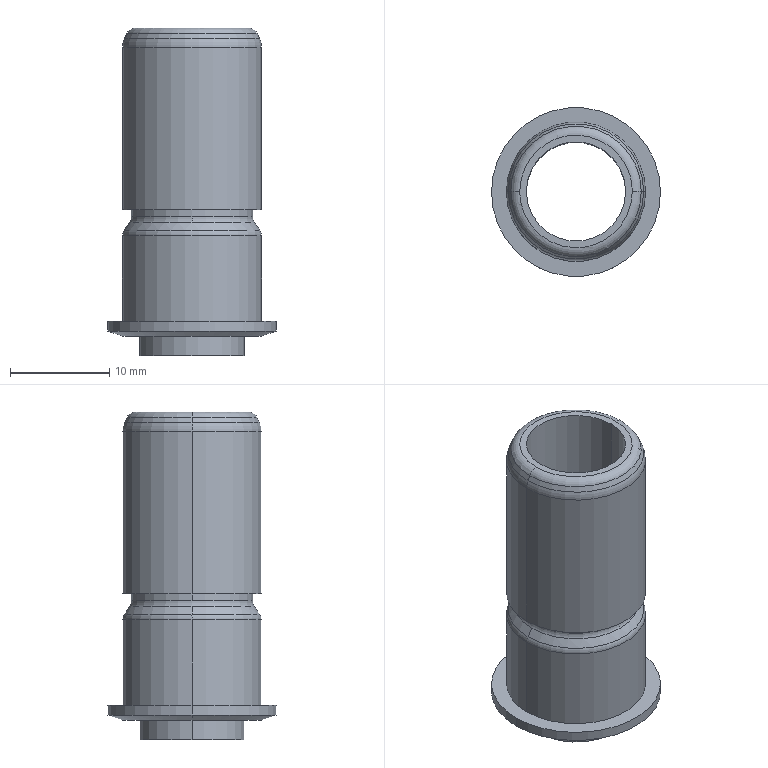Part | NX | features BREP 1 | 1 solid | 31 faces | box 17 x 17 x 33 mm | volume 2358 mm3 | cylinder 12 | torus 8 | cone 6 | plane 5 | commonest cylinder face diameters 14 x4 10 x2 10.5 x2 12.2 x2 17 x2
STEP:
#1=CARTESIAN_POINT('',(-514.52,233.142,1216.091));
#2=VERTEX_POINT('',#1);
#3=CARTESIAN_POINT('',(-524.52,233.142,1216.091));
#4=VERTEX_POINT('',#3);
#5=CARTESIAN_POINT('',(-519.52,233.142,1216.091));
#6=DIRECTION('',(0.,0.,-1.));
#7=DIRECTION('',(-1.,0.,0.));
#8=AXIS2_PLACEMENT_3D('',#5,#6,#7);
#9=CIRCLE('',#8,5.);
#10=EDGE_CURVE('',#2,#4,#9,.T.);
#11=ORIENTED_EDGE('',*,*,#10,.F.);
#12=CARTESIAN_POINT('',(-514.52,233.142,1183.091));
#13=VERTEX_POINT('',#12);
#14=CARTESIAN_POINT('',(-514.52,233.142,1216.091));
#15=DIRECTION('',(0.,0.,-1.));
#16=VECTOR('',#15,1000.);
#17=LINE('',#14,#16);
#18=EDGE_CURVE('',#13,#2,#17,.F.);
#19=ORIENTED_EDGE('',*,*,#18,.F.);
#20=CARTESIAN_POINT('',(-524.52,233.142,1183.091));
#21=VERTEX_POINT('',#20);
#22=CARTESIAN_POINT('',(-519.52,233.142,1183.091));
#23=DIRECTION('',(0.,0.,1.));
#24=DIRECTION('',(-1.,0.,0.));
#25=AXIS2_PLACEMENT_3D('',#22,#23,#24);
#26=CIRCLE('',#25,5.);
#27=EDGE_CURVE('',#21,#13,#26,.T.);
#28=ORIENTED_EDGE('',*,*,#27,.F.);
#29=CARTESIAN_POINT('',(-524.52,233.142,1216.091));
#30=DIRECTION('',(0.,0.,-1.));
#31=VECTOR('',#30,1000.);
#32=LINE('',#29,#31);
#33=EDGE_CURVE('',#21,#4,#32,.F.);
#34=ORIENTED_EDGE('',*,*,#33,.T.);
#35=EDGE_LOOP('',(#11,#19,#28,#34));
#36=FACE_BOUND('',#35,.T.);
#37=CARTESIAN_POINT('',(-519.52,233.142,1216.091));
#38=DIRECTION('',(0.,0.,-1.));
#39=DIRECTION('',(1.,0.,0.));
#40=AXIS2_PLACEMENT_3D('',#37,#38,#39);
#41=CYLINDRICAL_SURFACE('',#40,5.);
#42=ADVANCED_FACE('',(#36),#41,.F.);
#43=CARTESIAN_POINT('',(-512.95,233.142,1215.514));
#44=VERTEX_POINT('',#43);
#45=CARTESIAN_POINT('',(-526.089,233.142,1215.514));
#46=VERTEX_POINT('',#45);
#47=CARTESIAN_POINT('',(-519.52,233.142,1215.514));
#48=DIRECTION('',(0.,0.,1.));
#49=DIRECTION('',(0.01126,0.9999,0.));
#50=AXIS2_PLACEMENT_3D('',#47,#48,#49);
#51=CIRCLE('',#50,6.569);
#52=EDGE_CURVE('',#44,#46,#51,.T.);
#53=ORIENTED_EDGE('',*,*,#52,.T.);
#54=CARTESIAN_POINT('',(-525.182,233.142,1216.091));
#55=VERTEX_POINT('',#54);
#56=CARTESIAN_POINT('',(-525.182,233.142,1215.091));
#57=DIRECTION('',(0.,1.,0.));
#58=DIRECTION('',(0.,0.,1.));
#59=AXIS2_PLACEMENT_3D('',#56,#57,#58);
#60=CIRCLE('',#59,1.);
#61=EDGE_CURVE('',#46,#55,#60,.T.);
#62=ORIENTED_EDGE('',*,*,#61,.T.);
#63=CARTESIAN_POINT('',(-519.587,238.804,1216.091));
#64=VERTEX_POINT('',#63);
#65=CARTESIAN_POINT('',(-525.182,233.142,1216.091));
#66=CARTESIAN_POINT('',(-525.182,233.51,1216.091));
#67=CARTESIAN_POINT('',(-525.146,233.878,1216.091));
#68=CARTESIAN_POINT('',(-525.057,234.328,1216.091));
#69=CARTESIAN_POINT('',(-525.037,234.418,1216.091));
#70=CARTESIAN_POINT('',(-525.004,234.552,1216.091));
#71=CARTESIAN_POINT('',(-524.986,234.619,1216.091));
#72=CARTESIAN_POINT('',(-524.966,234.691,1216.091));
#73=CARTESIAN_POINT('',(-524.958,234.719,1216.091));
#74=CARTESIAN_POINT('',(-524.955,234.73,1216.091));
#75=CARTESIAN_POINT('',(-524.953,234.737,1216.091));
#76=CARTESIAN_POINT('',(-524.952,234.741,1216.091));
#77=CARTESIAN_POINT('',(-524.951,234.744,1216.091));
#78=CARTESIAN_POINT('',(-524.941,234.779,1216.091));
#79=CARTESIAN_POINT('',(-524.919,234.853,1216.091));
#80=CARTESIAN_POINT('',(-524.87,234.997,1216.091));
#81=CARTESIAN_POINT('',(-524.859,235.029,1216.091));
#82=CARTESIAN_POINT('',(-524.841,235.08,1216.091));
#83=CARTESIAN_POINT('',(-524.831,235.106,1216.091));
#84=CARTESIAN_POINT('',(-524.82,235.134,1216.091));
#85=CARTESIAN_POINT('',(-524.815,235.148,1216.091));
#86=CARTESIAN_POINT('',(-524.813,235.154,1216.091));
#87=CARTESIAN_POINT('',(-524.811,235.16,1216.091));
#88=CARTESIAN_POINT('',(-524.792,235.209,1216.091));
#89=CARTESIAN_POINT('',(-524.773,235.257,1216.091));
#90=CARTESIAN_POINT('',(-524.681,235.479,1216.091));
#91=CARTESIAN_POINT('',(-524.602,235.646,1216.091));
#92=CARTESIAN_POINT('',(-524.499,235.84,1216.091));
#93=CARTESIAN_POINT('',(-524.478,235.878,1216.091));
#94=CARTESIAN_POINT('',(-524.436,235.953,1216.091));
#95=CARTESIAN_POINT('',(-524.413,235.992,1216.091));
#96=CARTESIAN_POINT('',(-524.342,236.111,1216.091));
#97=CARTESIAN_POINT('',(-524.293,236.189,1216.091));
#98=CARTESIAN_POINT('',(-524.141,236.419,1216.091));
#99=CARTESIAN_POINT('',(-524.032,236.568,1216.091));
#100=CARTESIAN_POINT('',(-523.858,236.782,1216.091));
#101=CARTESIAN_POINT('',(-523.768,236.887,1216.091));
#102=CARTESIAN_POINT('',(-523.659,237.006,1216.091));
#103=CARTESIAN_POINT('',(-523.604,237.065,1216.091));
#104=CARTESIAN_POINT('',(-523.576,237.093,1216.091));
#105=CARTESIAN_POINT('',(-523.562,237.108,1216.091));
#106=CARTESIAN_POINT('',(-523.556,237.114,1216.091));
#107=CARTESIAN_POINT('',(-523.552,237.118,1216.091));
#108=CARTESIAN_POINT('',(-523.549,237.121,1216.091));
#109=CARTESIAN_POINT('',(-523.495,237.176,1216.091));
#110=CARTESIAN_POINT('',(-523.385,237.288,1216.091));
#111=CARTESIAN_POINT('',(-523.159,237.481,1216.091));
#112=CARTESIAN_POINT('',(-523.109,237.522,1216.091));
#113=CARTESIAN_POINT('',(-523.041,237.576,1216.091));
#114=CARTESIAN_POINT('',(-523.024,237.59,1216.091));
#115=CARTESIAN_POINT('',(-523.006,237.604,1216.091));
#116=CARTESIAN_POINT('',(-522.999,237.61,1216.091));
#117=CARTESIAN_POINT('',(-522.997,237.611,1216.091));
#118=CARTESIAN_POINT('',(-522.991,237.616,1216.091));
#119=CARTESIAN_POINT('',(-522.97,237.632,1216.091));
#120=CARTESIAN_POINT('',(-522.882,237.699,1216.091));
#121=CARTESIAN_POINT('',(-522.719,237.816,1216.091));
#122=CARTESIAN_POINT('',(-522.559,237.921,1216.091));
#123=CARTESIAN_POINT('',(-522.39,238.024,1216.091));
#124=CARTESIAN_POINT('',(-522.3,238.076,1216.091));
#125=CARTESIAN_POINT('',(-522.036,238.219,1216.091));
#126=CARTESIAN_POINT('',(-521.865,238.299,1216.091));
#127=CARTESIAN_POINT('',(-521.619,238.402,1216.091));
#128=CARTESIAN_POINT('',(-521.539,238.433,1216.091));
#129=CARTESIAN_POINT('',(-521.421,238.476,1216.091));
#130=CARTESIAN_POINT('',(-521.383,238.49,1216.091));
#131=CARTESIAN_POINT('',(-521.306,238.516,1216.091));
#132=CARTESIAN_POINT('',(-521.26,238.531,1216.091));
#133=CARTESIAN_POINT('',(-521.041,238.6,1216.091));
#134=CARTESIAN_POINT('',(-520.863,238.646,1216.091));
#135=CARTESIAN_POINT('',(-520.322,238.76,1216.091));
#136=CARTESIAN_POINT('',(-519.955,238.8,1216.091));
#137=CARTESIAN_POINT('',(-519.587,238.804,1216.091));
#138=B_SPLINE_CURVE_WITH_KNOTS('',3,(#65,#66,#67,#68,#69,#70,#71,#72,#73,#74,#75,#76,#77,#78,#79,#80,#81,#82,#83,#84,#85,#86,#87,#88,#89,#90,#91,#92,#93,#94,#95,#96,#97,#98,#99,#100,#101,#102,#103,#104,#105,#106,#107,#108,#109,#110,#111,#112,#113,#114,#115,#116,#117,#118,#119,#120,#121,#122,#123,#124,#125,#126,#127,#128,#129,#130,#131,#132,#133,#134,#135,#136,#137),.UNSPECIFIED.,.F.,.F.,(4,2,2,1,1,2,2,2,2,2,1,2,2,1,2,2,2,2,2,2,1,1,1,1,1,2,2,2,2,1,2,2,1,1,1,2,2,2,2,2,2,2,4),(0.,0.125,0.1562,0.1719,0.1797,0.1816,0.1836,0.1875,0.2187,0.2266,0.2305,0.2324,0.2334,0.2344,0.25,0.3125,0.3281,0.3438,0.375,0.4375,0.4688,0.4844,0.4922,0.4961,0.498,0.499,0.5,0.5625,0.5781,0.582,0.583,0.584,0.5859,0.5938,0.625,0.6563,0.6875,0.75,0.7813,0.7969,0.8125,0.875,1.),.UNSPECIFIED.);
#139=EDGE_CURVE('',#55,#64,#138,.T.);
#140=ORIENTED_EDGE('',*,*,#139,.T.);
#141=CARTESIAN_POINT('',(-519.456,238.804,1216.091));
#142=VERTEX_POINT('',#141);
#143=CARTESIAN_POINT('',(-519.587,238.804,1216.091));
#144=CARTESIAN_POINT('',(-519.543,238.805,1216.091));
#145=CARTESIAN_POINT('',(-519.499,238.805,1216.091));
#146=CARTESIAN_POINT('',(-519.456,238.804,1216.091));
#147=B_SPLINE_CURVE_WITH_KNOTS('',3,(#143,#144,#145,#146),.UNSPECIFIED.,.F.,.F.,(4,4),(0.,1.),.PIECEWISE_BEZIER_KNOTS.);
#148=EDGE_CURVE('',#64,#142,#147,.T.);
#149=ORIENTED_EDGE('',*,*,#148,.T.);
#150=CARTESIAN_POINT('',(-513.857,233.142,1216.091));
#151=VERTEX_POINT('',#150);
#152=CARTESIAN_POINT('',(-519.456,238.804,1216.091));
#153=CARTESIAN_POINT('',(-519.377,238.803,1216.091));
#154=CARTESIAN_POINT('',(-519.22,238.799,1216.091));
#155=CARTESIAN_POINT('',(-518.987,238.781,1216.091));
#156=CARTESIAN_POINT('',(-518.758,238.755,1216.091));
#157=CARTESIAN_POINT('',(-518.534,238.72,1216.091));
#158=CARTESIAN_POINT('',(-518.314,238.677,1216.091));
#159=CARTESIAN_POINT('',(-518.1,238.625,1216.091));
#160=CARTESIAN_POINT('',(-517.89,238.567,1216.091));
#161=CARTESIAN_POINT('',(-517.686,238.501,1216.091));
#162=CARTESIAN_POINT('',(-517.488,238.429,1216.091));
#163=CARTESIAN_POINT('',(-517.295,238.351,1216.091));
#164=CARTESIAN_POINT('',(-517.109,238.267,1216.091));
#165=CARTESIAN_POINT('',(-516.928,238.178,1216.091));
#166=CARTESIAN_POINT('',(-516.753,238.085,1216.091));
#167=CARTESIAN_POINT('',(-516.585,237.986,1216.091));
#168=CARTESIAN_POINT('',(-516.423,237.884,1216.091));
#169=CARTESIAN_POINT('',(-516.267,237.779,1216.091));
#170=CARTESIAN_POINT('',(-516.117,237.67,1216.091));
#171=CARTESIAN_POINT('',(-515.973,237.558,1216.091));
#172=CARTESIAN_POINT('',(-515.835,237.444,1216.091));
#173=CARTESIAN_POINT('',(-515.704,237.327,1216.091));
#174=CARTESIAN_POINT('',(-515.578,237.209,1216.091));
#175=CARTESIAN_POINT('',(-515.458,237.09,1216.091));
#176=CARTESIAN_POINT('',(-515.345,236.969,1216.091));
#177=CARTESIAN_POINT('',(-515.236,236.847,1216.091));
#178=CARTESIAN_POINT('',(-515.134,236.725,1216.091));
#179=CARTESIAN_POINT('',(-515.036,236.603,1216.091));
#180=CARTESIAN_POINT('',(-514.945,236.48,1216.091));
#181=CARTESIAN_POINT('',(-514.858,236.358,1216.091));
#182=CARTESIAN_POINT('',(-514.776,236.236,1216.091));
#183=CARTESIAN_POINT('',(-514.699,236.115,1216.091));
#184=CARTESIAN_POINT('',(-514.627,235.995,1216.091));
#185=CARTESIAN_POINT('',(-514.56,235.876,1216.091));
#186=CARTESIAN_POINT('',(-514.496,235.758,1216.091));
#187=CARTESIAN_POINT('',(-514.438,235.641,1216.091));
#188=CARTESIAN_POINT('',(-514.383,235.526,1216.091));
#189=CARTESIAN_POINT('',(-514.332,235.413,1216.091));
#190=CARTESIAN_POINT('',(-514.284,235.302,1216.091));
#191=CARTESIAN_POINT('',(-514.241,235.193,1216.091));
#192=CARTESIAN_POINT('',(-514.2,235.085,1216.091));
#193=CARTESIAN_POINT('',(-514.163,234.98,1216.091));
#194=CARTESIAN_POINT('',(-514.129,234.878,1216.091));
#195=CARTESIAN_POINT('',(-514.098,234.778,1216.091));
#196=CARTESIAN_POINT('',(-514.069,234.68,1216.091));
#197=CARTESIAN_POINT('',(-514.043,234.585,1216.091));
#198=CARTESIAN_POINT('',(-514.02,234.493,1216.091));
#199=CARTESIAN_POINT('',(-513.999,234.404,1216.091));
#200=CARTESIAN_POINT('',(-513.98,234.317,1216.091));
#201=CARTESIAN_POINT('',(-513.963,234.233,1216.091));
#202=CARTESIAN_POINT('',(-513.947,234.152,1216.091));
#203=CARTESIAN_POINT('',(-513.934,234.074,1216.091));
#204=CARTESIAN_POINT('',(-513.922,233.999,1216.091));
#205=CARTESIAN_POINT('',(-513.911,233.927,1216.091));
#206=CARTESIAN_POINT('',(-513.902,233.858,1216.091));
#207=CARTESIAN_POINT('',(-513.894,233.793,1216.091));
#208=CARTESIAN_POINT('',(-513.887,233.73,1216.091));
#209=CARTESIAN_POINT('',(-513.881,233.671,1216.091));
#210=CARTESIAN_POINT('',(-513.876,233.614,1216.091));
#211=CARTESIAN_POINT('',(-513.872,233.561,1216.091));
#212=CARTESIAN_POINT('',(-513.869,233.511,1216.091));
#213=CARTESIAN_POINT('',(-513.866,233.464,1216.091));
#214=CARTESIAN_POINT('',(-513.863,233.42,1216.091));
#215=CARTESIAN_POINT('',(-513.862,233.38,1216.091));
#216=CARTESIAN_POINT('',(-513.86,233.343,1216.091));
#217=CARTESIAN_POINT('',(-513.859,233.309,1216.091));
#218=CARTESIAN_POINT('',(-513.858,233.278,1216.091));
#219=CARTESIAN_POINT('',(-513.858,233.25,1216.091));
#220=CARTESIAN_POINT('',(-513.857,233.226,1216.091));
#221=CARTESIAN_POINT('',(-513.857,233.204,1216.091));
#222=CARTESIAN_POINT('',(-513.857,233.186,1216.091));
#223=CARTESIAN_POINT('',(-513.857,233.172,1216.091));
#224=CARTESIAN_POINT('',(-513.857,233.16,1216.091));
#225=CARTESIAN_POINT('',(-513.857,233.152,1216.091));
#226=CARTESIAN_POINT('',(-513.857,233.147,1216.091));
#227=CARTESIAN_POINT('',(-513.857,233.144,1216.091));
#228=CARTESIAN_POINT('',(-513.857,233.143,1216.091));
#229=CARTESIAN_POINT('',(-513.857,233.142,1216.091));
#230=B_SPLINE_CURVE_WITH_KNOTS('',3,(#152,#153,#154,#155,#156,#157,#158,#159,#160,#161,#162,#163,#164,#165,#166,#167,#168,#169,#170,#171,#172,#173,#174,#175,#176,#177,#178,#179,#180,#181,#182,#183,#184,#185,#186,#187,#188,#189,#190,#191,#192,#193,#194,#195,#196,#197,#198,#199,#200,#201,#202,#203,#204,#205,#206,#207,#208,#209,#210,#211,#212,#213,#214,#215,#216,#217,#218,#219,#220,#221,#222,#223,#224,#225,#226,#227,#228,#229),.UNSPECIFIED.,.F.,.F.,(4,1,1,1,1,1,1,1,1,1,1,1,1,1,1,1,1,1,1,1,1,1,1,1,1,1,1,1,1,1,1,1,1,1,1,1,1,1,1,1,1,1,1,1,1,1,1,1,1,1,1,1,1,1,1,1,1,1,1,1,1,1,1,1,1,1,1,1,1,1,1,1,1,1,1,4),(0.,0.0268,0.05324,0.07932,0.105,0.1304,0.1554,0.18,0.2042,0.2281,0.2517,0.2748,0.2976,0.3201,0.3421,0.3638,0.3852,0.4061,0.4268,0.447,0.4669,0.4864,0.5056,0.5244,0.5428,0.5609,0.5786,0.5959,0.6129,0.6295,0.6457,0.6616,0.6771,0.6923,0.707,0.7215,0.7355,0.7492,0.7625,0.7755,0.7881,0.8003,0.8122,0.8237,0.8349,0.8456,0.8561,0.8661,0.8758,0.8851,0.8941,0.9027,0.9109,0.9188,0.9263,0.9334,0.9402,0.9466,0.9526,0.9583,0.9636,0.9686,0.9732,0.9774,0.9812,0.9847,0.9879,0.9906,0.993,0.9951,0.9968,0.9981,0.999,0.9996,0.9998,1.),.UNSPECIFIED.);
#231=EDGE_CURVE('',#142,#151,#230,.T.);
#232=ORIENTED_EDGE('',*,*,#231,.T.);
#233=CARTESIAN_POINT('',(-513.857,233.142,1215.091));
#234=DIRECTION('',(0.,-1.,0.));
#235=DIRECTION('',(0.,0.,-1.));
#236=AXIS2_PLACEMENT_3D('',#233,#234,#235);
#237=CIRCLE('',#236,1.);
#238=EDGE_CURVE('',#44,#151,#237,.T.);
#239=ORIENTED_EDGE('',*,*,#238,.F.);
#240=EDGE_LOOP('',(#53,#62,#140,#149,#232,#239));
#241=FACE_BOUND('',#240,.T.);
#242=CARTESIAN_POINT('',(-519.52,233.142,1215.091));
#243=DIRECTION('',(0.,0.,1.));
#244=DIRECTION('',(-1.,0.,0.));
#245=AXIS2_PLACEMENT_3D('',#242,#243,#244);
#246=TOROIDAL_SURFACE('',#245,5.663,1.);
#247=ADVANCED_FACE('',(#241),#246,.T.);
#248=CARTESIAN_POINT('',(-524.77,233.142,1185.091));
#249=VERTEX_POINT('',#248);
#250=CARTESIAN_POINT('',(-514.27,233.142,1185.091));
#251=VERTEX_POINT('',#250);
#252=CARTESIAN_POINT('',(-519.52,233.142,1185.091));
#253=DIRECTION('',(0.,0.,-1.));
#254=DIRECTION('',(-1.,0.,0.));
#255=AXIS2_PLACEMENT_3D('',#252,#253,#254);
#256=CIRCLE('',#255,5.25);
#257=EDGE_CURVE('',#249,#251,#256,.T.);
#258=ORIENTED_EDGE('',*,*,#257,.T.);
#259=CARTESIAN_POINT('',(-514.27,233.142,1183.091));
#260=VERTEX_POINT('',#259);
#261=CARTESIAN_POINT('',(-514.27,233.142,1182.091));
#262=DIRECTION('',(0.,0.,-1.));
#263=VECTOR('',#262,1000.);
#264=LINE('',#261,#263);
#265=EDGE_CURVE('',#260,#251,#264,.F.);
#266=ORIENTED_EDGE('',*,*,#265,.F.);
#267=CARTESIAN_POINT('',(-524.77,233.142,1183.091));
#268=VERTEX_POINT('',#267);
#269=CARTESIAN_POINT('',(-519.52,233.142,1183.091));
#270=DIRECTION('',(0.,0.,-1.));
#271=DIRECTION('',(-1.,0.,0.));
#272=AXIS2_PLACEMENT_3D('',#269,#270,#271);
#273=CIRCLE('',#272,5.25);
#274=EDGE_CURVE('',#268,#260,#273,.T.);
#275=ORIENTED_EDGE('',*,*,#274,.F.);
#276=CARTESIAN_POINT('',(-524.77,233.142,1182.091));
#277=DIRECTION('',(0.,0.,-1.));
#278=VECTOR('',#277,1000.);
#279=LINE('',#276,#278);
#280=EDGE_CURVE('',#268,#249,#279,.F.);
#281=ORIENTED_EDGE('',*,*,#280,.T.);
#282=EDGE_LOOP('',(#258,#266,#275,#281));
#283=FACE_BOUND('',#282,.T.);
#284=CARTESIAN_POINT('',(-519.52,233.142,1182.091));
#285=DIRECTION('',(0.,0.,-1.));
#286=DIRECTION('',(1.,0.,0.));
#287=AXIS2_PLACEMENT_3D('',#284,#285,#286);
#288=CYLINDRICAL_SURFACE('',#287,5.25);
#289=ADVANCED_FACE('',(#283),#288,.T.);
#290=ORIENTED_EDGE('',*,*,#52,.F.);
#291=CARTESIAN_POINT('',(-512.707,233.142,1214.992));
#292=VERTEX_POINT('',#291);
#293=CARTESIAN_POINT('',(-512.707,233.142,1214.992));
#294=DIRECTION('',(0.4226,0.,-0.9063));
#295=VECTOR('',#294,1000.);
#296=LINE('',#293,#295);
#297=EDGE_CURVE('',#292,#44,#296,.F.);
#298=ORIENTED_EDGE('',*,*,#297,.F.);
#299=CARTESIAN_POINT('',(-526.332,233.142,1214.992));
#300=VERTEX_POINT('',#299);
#301=CARTESIAN_POINT('',(-519.52,233.142,1214.992));
#302=DIRECTION('',(0.,0.,1.));
#303=DIRECTION('',(-1.,0.,0.));
#304=AXIS2_PLACEMENT_3D('',#301,#302,#303);
#305=CIRCLE('',#304,6.813);
#306=EDGE_CURVE('',#292,#300,#305,.T.);
#307=ORIENTED_EDGE('',*,*,#306,.T.);
#308=CARTESIAN_POINT('',(-526.332,233.142,1214.992));
#309=DIRECTION('',(-0.4226,0.,-0.9063));
#310=VECTOR('',#309,1000.);
#311=LINE('',#308,#310);
#312=EDGE_CURVE('',#300,#46,#311,.F.);
#313=ORIENTED_EDGE('',*,*,#312,.T.);
#314=EDGE_LOOP('',(#290,#298,#307,#313));
#315=FACE_BOUND('',#314,.T.);
#316=CARTESIAN_POINT('',(-519.52,233.142,1214.992));
#317=DIRECTION('',(0.,0.,-1.));
#318=DIRECTION('',(1.,0.,0.));
#319=AXIS2_PLACEMENT_3D('',#316,#317,#318);
#320=CONICAL_SURFACE('',#319,6.813,0.4363);
#321=ADVANCED_FACE('',(#315),#320,.T.);
#322=CARTESIAN_POINT('',(-512.52,233.142,1214.146));
#323=VERTEX_POINT('',#322);
#324=CARTESIAN_POINT('',(-526.52,233.142,1214.146));
#325=VERTEX_POINT('',#324);
#326=CARTESIAN_POINT('',(-519.52,233.142,1214.146));
#327=DIRECTION('',(0.,0.,1.));
#328=DIRECTION('',(0.007772,-1.,0.));
#329=AXIS2_PLACEMENT_3D('',#326,#327,#328);
#330=CIRCLE('',#329,7.);
#331=EDGE_CURVE('',#323,#325,#330,.T.);
#332=ORIENTED_EDGE('',*,*,#331,.T.);
#333=CARTESIAN_POINT('',(-524.52,233.142,1214.146));
#334=DIRECTION('',(0.,1.,0.));
#335=DIRECTION('',(-1.,0.,0.));
#336=AXIS2_PLACEMENT_3D('',#333,#334,#335);
#337=CIRCLE('',#336,2.);
#338=EDGE_CURVE('',#325,#300,#337,.T.);
#339=ORIENTED_EDGE('',*,*,#338,.T.);
#340=ORIENTED_EDGE('',*,*,#306,.F.);
#341=CARTESIAN_POINT('',(-514.52,233.142,1214.146));
#342=DIRECTION('',(0.,-1.,0.));
#343=DIRECTION('',(0.,0.,-1.));
#344=AXIS2_PLACEMENT_3D('',#341,#342,#343);
#345=CIRCLE('',#344,2.);
#346=EDGE_CURVE('',#323,#292,#345,.T.);
#347=ORIENTED_EDGE('',*,*,#346,.F.);
#348=EDGE_LOOP('',(#332,#339,#340,#347));
#349=FACE_BOUND('',#348,.T.);
#350=CARTESIAN_POINT('',(-519.52,233.142,1214.146));
#351=DIRECTION('',(0.,0.,1.));
#352=DIRECTION('',(-1.,0.,0.));
#353=AXIS2_PLACEMENT_3D('',#350,#351,#352);
#354=TOROIDAL_SURFACE('',#353,5.,2.);
#355=ADVANCED_FACE('',(#349),#354,.T.);
#356=CARTESIAN_POINT('',(-526.52,233.142,1185.091));
#357=VERTEX_POINT('',#356);
#358=CARTESIAN_POINT('',(-512.52,233.142,1185.091));
#359=VERTEX_POINT('',#358);
#360=CARTESIAN_POINT('',(-519.52,233.142,1185.091));
#361=DIRECTION('',(0.,0.,-1.));
#362=DIRECTION('',(1.,0.,0.));
#363=AXIS2_PLACEMENT_3D('',#360,#361,#362);
#364=CIRCLE('',#363,7.);
#365=EDGE_CURVE('',#357,#359,#364,.T.);
#366=ORIENTED_EDGE('',*,*,#365,.F.);
#367=CARTESIAN_POINT('',(-528.02,233.142,1185.591));
#368=VERTEX_POINT('',#367);
#369=CARTESIAN_POINT('',(-528.02,233.142,1185.591));
#370=DIRECTION('',(-0.9487,0.,0.3162));
#371=VECTOR('',#370,1000.);
#372=LINE('',#369,#371);
#373=EDGE_CURVE('',#357,#368,#372,.T.);
#374=ORIENTED_EDGE('',*,*,#373,.T.);
#375=CARTESIAN_POINT('',(-511.02,233.142,1185.591));
#376=VERTEX_POINT('',#375);
#377=CARTESIAN_POINT('',(-519.52,233.142,1185.591));
#378=DIRECTION('',(0.,0.,-1.));
#379=DIRECTION('',(1.,0.,0.));
#380=AXIS2_PLACEMENT_3D('',#377,#378,#379);
#381=CIRCLE('',#380,8.5);
#382=EDGE_CURVE('',#368,#376,#381,.T.);
#383=ORIENTED_EDGE('',*,*,#382,.T.);
#384=CARTESIAN_POINT('',(-511.02,233.142,1185.591));
#385=DIRECTION('',(0.9487,0.,0.3162));
#386=VECTOR('',#385,1000.);
#387=LINE('',#384,#386);
#388=EDGE_CURVE('',#359,#376,#387,.T.);
#389=ORIENTED_EDGE('',*,*,#388,.F.);
#390=EDGE_LOOP('',(#366,#374,#383,#389));
#391=FACE_BOUND('',#390,.T.);
#392=CARTESIAN_POINT('',(-519.52,233.142,1185.591));
#393=DIRECTION('',(0.,0.,1.));
#394=DIRECTION('',(-1.,0.,0.));
#395=AXIS2_PLACEMENT_3D('',#392,#393,#394);
#396=CONICAL_SURFACE('',#395,8.5,1.249);
#397=ADVANCED_FACE('',(#391),#396,.T.);
#398=ORIENTED_EDGE('',*,*,#331,.F.);
#399=CARTESIAN_POINT('',(-512.52,233.142,1197.791));
#400=VERTEX_POINT('',#399);
#401=CARTESIAN_POINT('',(-512.52,233.142,1216.091));
#402=DIRECTION('',(0.,0.,-1.));
#403=VECTOR('',#402,1000.);
#404=LINE('',#401,#403);
#405=EDGE_CURVE('',#400,#323,#404,.F.);
#406=ORIENTED_EDGE('',*,*,#405,.F.);
#407=CARTESIAN_POINT('',(-526.52,233.142,1197.791));
#408=VERTEX_POINT('',#407);
#409=CARTESIAN_POINT('',(-519.52,233.142,1197.791));
#410=DIRECTION('',(0.,0.,1.));
#411=DIRECTION('',(-1.,0.,0.));
#412=AXIS2_PLACEMENT_3D('',#409,#410,#411);
#413=CIRCLE('',#412,7.);
#414=EDGE_CURVE('',#400,#408,#413,.T.);
#415=ORIENTED_EDGE('',*,*,#414,.T.);
#416=CARTESIAN_POINT('',(-526.52,233.142,1216.091));
#417=DIRECTION('',(0.,0.,-1.));
#418=VECTOR('',#417,1000.);
#419=LINE('',#416,#418);
#420=EDGE_CURVE('',#408,#325,#419,.F.);
#421=ORIENTED_EDGE('',*,*,#420,.T.);
#422=EDGE_LOOP('',(#398,#406,#415,#421));
#423=FACE_BOUND('',#422,.T.);
#424=CARTESIAN_POINT('',(-519.52,233.142,1216.091));
#425=DIRECTION('',(0.,0.,-1.));
#426=DIRECTION('',(1.,0.,0.));
#427=AXIS2_PLACEMENT_3D('',#424,#425,#426);
#428=CYLINDRICAL_SURFACE('',#427,7.);
#429=ADVANCED_FACE('',(#423),#428,.T.);
#430=CARTESIAN_POINT('',(-528.02,233.142,1186.591));
#431=VERTEX_POINT('',#430);
#432=CARTESIAN_POINT('',(-511.02,233.142,1186.591));
#433=VERTEX_POINT('',#432);
#434=CARTESIAN_POINT('',(-519.52,233.142,1186.591));
#435=DIRECTION('',(0.,0.,-1.));
#436=DIRECTION('',(-1.,0.,0.));
#437=AXIS2_PLACEMENT_3D('',#434,#435,#436);
#438=CIRCLE('',#437,8.5);
#439=EDGE_CURVE('',#431,#433,#438,.T.);
#440=ORIENTED_EDGE('',*,*,#439,.T.);
#441=CARTESIAN_POINT('',(-511.02,233.142,1216.091));
#442=DIRECTION('',(0.,0.,-1.));
#443=VECTOR('',#442,1000.);
#444=LINE('',#441,#443);
#445=EDGE_CURVE('',#376,#433,#444,.F.);
#446=ORIENTED_EDGE('',*,*,#445,.F.);
#447=ORIENTED_EDGE('',*,*,#382,.F.);
#448=CARTESIAN_POINT('',(-528.02,233.142,1216.091));
#449=DIRECTION('',(0.,0.,-1.));
#450=VECTOR('',#449,1000.);
#451=LINE('',#448,#450);
#452=EDGE_CURVE('',#368,#431,#451,.F.);
#453=ORIENTED_EDGE('',*,*,#452,.T.);
#454=EDGE_LOOP('',(#440,#446,#447,#453));
#455=FACE_BOUND('',#454,.T.);
#456=CARTESIAN_POINT('',(-519.52,233.142,1216.091));
#457=DIRECTION('',(0.,0.,-1.));
#458=DIRECTION('',(1.,0.,0.));
#459=AXIS2_PLACEMENT_3D('',#456,#457,#458);
#460=CYLINDRICAL_SURFACE('',#459,8.5);
#461=ADVANCED_FACE('',(#455),#460,.T.);
#462=CARTESIAN_POINT('',(-513.42,233.142,1197.791));
#463=VERTEX_POINT('',#462);
#464=CARTESIAN_POINT('',(-525.62,233.142,1197.791));
#465=VERTEX_POINT('',#464);
#466=CARTESIAN_POINT('',(-519.52,233.142,1197.791));
#467=DIRECTION('',(0.,0.,1.));
#468=DIRECTION('',(-1.,0.,0.));
#469=AXIS2_PLACEMENT_3D('',#466,#467,#468);
#470=CIRCLE('',#469,6.1);
#471=EDGE_CURVE('',#463,#465,#470,.T.);
#472=ORIENTED_EDGE('',*,*,#471,.F.);
#473=CARTESIAN_POINT('',(-513.42,233.142,1197.103));
#474=VERTEX_POINT('',#473);
#475=CARTESIAN_POINT('',(-513.42,233.142,1216.091));
#476=DIRECTION('',(0.,0.,-1.));
#477=VECTOR('',#476,1000.);
#478=LINE('',#475,#477);
#479=EDGE_CURVE('',#474,#463,#478,.F.);
#480=ORIENTED_EDGE('',*,*,#479,.F.);
#481=CARTESIAN_POINT('',(-519.52,239.242,1197.103));
#482=VERTEX_POINT('',#481);
#483=CARTESIAN_POINT('',(-519.52,233.142,1197.103));
#484=DIRECTION('',(0.,0.,1.));
#485=DIRECTION('',(-1.,0.,0.));
#486=AXIS2_PLACEMENT_3D('',#483,#484,#485);
#487=CIRCLE('',#486,6.1);
#488=EDGE_CURVE('',#474,#482,#487,.T.);
#489=ORIENTED_EDGE('',*,*,#488,.T.);
#490=CARTESIAN_POINT('',(-525.62,233.142,1197.103));
#491=VERTEX_POINT('',#490);
#492=CARTESIAN_POINT('',(-519.52,233.142,1197.103));
#493=DIRECTION('',(0.,0.,1.));
#494=DIRECTION('',(-1.,0.,0.));
#495=AXIS2_PLACEMENT_3D('',#492,#493,#494);
#496=CIRCLE('',#495,6.1);
#497=EDGE_CURVE('',#482,#491,#496,.T.);
#498=ORIENTED_EDGE('',*,*,#497,.T.);
#499=CARTESIAN_POINT('',(-525.62,233.142,1216.091));
#500=DIRECTION('',(0.,0.,-1.));
#501=VECTOR('',#500,1000.);
#502=LINE('',#499,#501);
#503=EDGE_CURVE('',#491,#465,#502,.F.);
#504=ORIENTED_EDGE('',*,*,#503,.T.);
#505=EDGE_LOOP('',(#472,#480,#489,#498,#504));
#506=FACE_BOUND('',#505,.T.);
#507=CARTESIAN_POINT('',(-519.52,233.142,1216.091));
#508=DIRECTION('',(0.,0.,-1.));
#509=DIRECTION('',(1.,0.,0.));
#510=AXIS2_PLACEMENT_3D('',#507,#508,#509);
#511=CYLINDRICAL_SURFACE('',#510,6.1);
#512=ADVANCED_FACE('',(#506),#511,.T.);
#513=CARTESIAN_POINT('',(-526.52,233.142,1195.179));
#514=VERTEX_POINT('',#513);
#515=CARTESIAN_POINT('',(-512.52,233.142,1195.179));
#516=VERTEX_POINT('',#515);
#517=CARTESIAN_POINT('',(-519.52,233.142,1195.179));
#518=DIRECTION('',(0.,0.,-1.));
#519=DIRECTION('',(-1.,0.,0.));
#520=AXIS2_PLACEMENT_3D('',#517,#518,#519);
#521=CIRCLE('',#520,7.);
#522=EDGE_CURVE('',#514,#516,#521,.T.);
#523=ORIENTED_EDGE('',*,*,#522,.T.);
#524=CARTESIAN_POINT('',(-512.52,233.142,1186.591));
#525=VERTEX_POINT('',#524);
#526=CARTESIAN_POINT('',(-512.52,233.142,1216.091));
#527=DIRECTION('',(0.,0.,-1.));
#528=VECTOR('',#527,1000.);
#529=LINE('',#526,#528);
#530=EDGE_CURVE('',#525,#516,#529,.F.);
#531=ORIENTED_EDGE('',*,*,#530,.F.);
#532=CARTESIAN_POINT('',(-526.52,233.142,1186.591));
#533=VERTEX_POINT('',#532);
#534=CARTESIAN_POINT('',(-519.52,233.142,1186.591));
#535=DIRECTION('',(0.,0.,-1.));
#536=DIRECTION('',(-1.,0.,0.));
#537=AXIS2_PLACEMENT_3D('',#534,#535,#536);
#538=CIRCLE('',#537,7.);
#539=EDGE_CURVE('',#533,#525,#538,.T.);
#540=ORIENTED_EDGE('',*,*,#539,.F.);
#541=CARTESIAN_POINT('',(-526.52,233.142,1216.091));
#542=DIRECTION('',(0.,0.,-1.));
#543=VECTOR('',#542,1000.);
#544=LINE('',#541,#543);
#545=EDGE_CURVE('',#533,#514,#544,.F.);
#546=ORIENTED_EDGE('',*,*,#545,.T.);
#547=EDGE_LOOP('',(#523,#531,#540,#546));
#548=FACE_BOUND('',#547,.T.);
#549=CARTESIAN_POINT('',(-519.52,233.142,1216.091));
#550=DIRECTION('',(0.,0.,-1.));
#551=DIRECTION('',(1.,0.,0.));
#552=AXIS2_PLACEMENT_3D('',#549,#550,#551);
#553=CYLINDRICAL_SURFACE('',#552,7.);
#554=ADVANCED_FACE('',(#548),#553,.T.);
#555=CARTESIAN_POINT('',(-519.52,226.864,1196.534));
#556=VERTEX_POINT('',#555);
#557=CARTESIAN_POINT('',(-525.797,233.142,1196.534));
#558=VERTEX_POINT('',#557);
#559=CARTESIAN_POINT('',(-519.52,233.142,1196.534));
#560=DIRECTION('',(0.,0.,-1.));
#561=DIRECTION('',(0.00805,-1.,0.));
#562=AXIS2_PLACEMENT_3D('',#559,#560,#561);
#563=CIRCLE('',#562,6.278);
#564=EDGE_CURVE('',#556,#558,#563,.T.);
#565=ORIENTED_EDGE('',*,*,#564,.F.);
#566=CARTESIAN_POINT('',(-519.52,227.042,1197.103));
#567=VERTEX_POINT('',#566);
#568=CARTESIAN_POINT('',(-519.52,226.042,1197.103));
#569=DIRECTION('',(1.,0.,0.));
#570=DIRECTION('',(0.,0.,-1.));
#571=AXIS2_PLACEMENT_3D('',#568,#569,#570);
#572=CIRCLE('',#571,1.);
#573=EDGE_CURVE('',#556,#567,#572,.T.);
#574=ORIENTED_EDGE('',*,*,#573,.T.);
#575=CARTESIAN_POINT('',(-519.52,233.142,1197.103));
#576=DIRECTION('',(0.,0.,1.));
#577=DIRECTION('',(-1.,0.,0.));
#578=AXIS2_PLACEMENT_3D('',#575,#576,#577);
#579=CIRCLE('',#578,6.1);
#580=EDGE_CURVE('',#491,#567,#579,.T.);
#581=ORIENTED_EDGE('',*,*,#580,.F.);
#582=ORIENTED_EDGE('',*,*,#497,.F.);
#583=CARTESIAN_POINT('',(-519.52,239.42,1196.534));
#584=VERTEX_POINT('',#583);
#585=CARTESIAN_POINT('',(-519.52,240.242,1197.103));
#586=DIRECTION('',(-1.,0.,0.));
#587=DIRECTION('',(0.,0.,1.));
#588=AXIS2_PLACEMENT_3D('',#585,#586,#587);
#589=CIRCLE('',#588,1.);
#590=EDGE_CURVE('',#584,#482,#589,.T.);
#591=ORIENTED_EDGE('',*,*,#590,.F.);
#592=CARTESIAN_POINT('',(-519.52,233.142,1196.534));
#593=DIRECTION('',(0.,0.,-1.));
#594=DIRECTION('',(0.00805,-1.,0.));
#595=AXIS2_PLACEMENT_3D('',#592,#593,#594);
#596=CIRCLE('',#595,6.278);
#597=EDGE_CURVE('',#558,#584,#596,.T.);
#598=ORIENTED_EDGE('',*,*,#597,.F.);
#599=EDGE_LOOP('',(#565,#574,#581,#582,#591,#598));
#600=FACE_BOUND('',#599,.T.);
#601=CARTESIAN_POINT('',(-519.52,233.142,1197.103));
#602=DIRECTION('',(0.,0.,-1.));
#603=DIRECTION('',(0.,-1.,0.));
#604=AXIS2_PLACEMENT_3D('',#601,#602,#603);
#605=TOROIDAL_SURFACE('',#604,7.1,1.);
#606=ADVANCED_FACE('',(#600),#605,.F.);
#607=ORIENTED_EDGE('',*,*,#522,.F.);
#608=CARTESIAN_POINT('',(-526.342,233.142,1195.748));
#609=VERTEX_POINT('',#608);
#610=CARTESIAN_POINT('',(-525.52,233.142,1195.179));
#611=DIRECTION('',(0.,1.,0.));
#612=DIRECTION('',(0.,0.,1.));
#613=AXIS2_PLACEMENT_3D('',#610,#611,#612);
#614=CIRCLE('',#613,1.);
#615=EDGE_CURVE('',#514,#609,#614,.T.);
#616=ORIENTED_EDGE('',*,*,#615,.T.);
#617=CARTESIAN_POINT('',(-512.697,233.142,1195.748));
#618=VERTEX_POINT('',#617);
#619=CARTESIAN_POINT('',(-519.52,233.142,1195.748));
#620=DIRECTION('',(0.,0.,-1.));
#621=DIRECTION('',(-0.007896,1.,0.));
#622=AXIS2_PLACEMENT_3D('',#619,#620,#621);
#623=CIRCLE('',#622,6.822);
#624=EDGE_CURVE('',#609,#618,#623,.T.);
#625=ORIENTED_EDGE('',*,*,#624,.T.);
#626=CARTESIAN_POINT('',(-513.52,233.142,1195.179));
#627=DIRECTION('',(0.,-1.,0.));
#628=DIRECTION('',(0.,0.,-1.));
#629=AXIS2_PLACEMENT_3D('',#626,#627,#628);
#630=CIRCLE('',#629,1.);
#631=EDGE_CURVE('',#516,#618,#630,.T.);
#632=ORIENTED_EDGE('',*,*,#631,.F.);
#633=EDGE_LOOP('',(#607,#616,#625,#632));
#634=FACE_BOUND('',#633,.T.);
#635=CARTESIAN_POINT('',(-519.52,233.142,1195.179));
#636=DIRECTION('',(0.,0.,1.));
#637=DIRECTION('',(-1.,0.,0.));
#638=AXIS2_PLACEMENT_3D('',#635,#636,#637);
#639=TOROIDAL_SURFACE('',#638,6.,1.);
#640=ADVANCED_FACE('',(#634),#639,.T.);
#641=ORIENTED_EDGE('',*,*,#597,.T.);
#642=CARTESIAN_POINT('',(-513.242,233.142,1196.534));
#643=VERTEX_POINT('',#642);
#644=CARTESIAN_POINT('',(-519.52,233.142,1196.534));
#645=DIRECTION('',(0.,0.,-1.));
#646=DIRECTION('',(0.00805,-1.,0.));
#647=AXIS2_PLACEMENT_3D('',#644,#645,#646);
#648=CIRCLE('',#647,6.278);
#649=EDGE_CURVE('',#584,#643,#648,.T.);
#650=ORIENTED_EDGE('',*,*,#649,.T.);
#651=CARTESIAN_POINT('',(-512.697,233.142,1195.748));
#652=DIRECTION('',(0.5692,0.,-0.8222));
#653=VECTOR('',#652,1000.);
#654=LINE('',#651,#653);
#655=EDGE_CURVE('',#618,#643,#654,.F.);
#656=ORIENTED_EDGE('',*,*,#655,.F.);
#657=ORIENTED_EDGE('',*,*,#624,.F.);
#658=CARTESIAN_POINT('',(-526.342,233.142,1195.748));
#659=DIRECTION('',(-0.5692,0.,-0.8222));
#660=VECTOR('',#659,1000.);
#661=LINE('',#658,#660);
#662=EDGE_CURVE('',#609,#558,#661,.F.);
#663=ORIENTED_EDGE('',*,*,#662,.T.);
#664=EDGE_LOOP('',(#641,#650,#656,#657,#663));
#665=FACE_BOUND('',#664,.T.);
#666=CARTESIAN_POINT('',(-519.52,233.142,1195.748));
#667=DIRECTION('',(0.,0.,-1.));
#668=DIRECTION('',(1.,0.,0.));
#669=AXIS2_PLACEMENT_3D('',#666,#667,#668);
#670=CONICAL_SURFACE('',#669,6.822,0.6055);
#671=ADVANCED_FACE('',(#665),#670,.T.);
#672=ORIENTED_EDGE('',*,*,#18,.T.);
#673=CARTESIAN_POINT('',(-519.52,233.142,1216.091));
#674=DIRECTION('',(0.,0.,-1.));
#675=DIRECTION('',(-1.,0.,0.));
#676=AXIS2_PLACEMENT_3D('',#673,#674,#675);
#677=CIRCLE('',#676,5.);
#678=EDGE_CURVE('',#4,#2,#677,.T.);
#679=ORIENTED_EDGE('',*,*,#678,.F.);
#680=ORIENTED_EDGE('',*,*,#33,.F.);
#681=CARTESIAN_POINT('',(-519.52,233.142,1183.091));
#682=DIRECTION('',(0.,0.,1.));
#683=DIRECTION('',(-1.,0.,0.));
#684=AXIS2_PLACEMENT_3D('',#681,#682,#683);
#685=CIRCLE('',#684,5.);
#686=EDGE_CURVE('',#13,#21,#685,.T.);
#687=ORIENTED_EDGE('',*,*,#686,.F.);
#688=EDGE_LOOP('',(#672,#679,#680,#687));
#689=FACE_BOUND('',#688,.T.);
#690=CARTESIAN_POINT('',(-519.52,233.142,1216.091));
#691=DIRECTION('',(0.,0.,-1.));
#692=DIRECTION('',(1.,0.,0.));
#693=AXIS2_PLACEMENT_3D('',#690,#691,#692);
#694=CYLINDRICAL_SURFACE('',#693,5.);
#695=ADVANCED_FACE('',(#689),#694,.F.);
#696=CARTESIAN_POINT('',(-519.583,227.479,1216.091));
#697=VERTEX_POINT('',#696);
#698=CARTESIAN_POINT('',(-519.583,227.479,1216.091));
#699=CARTESIAN_POINT('',(-519.598,227.48,1216.091));
#700=CARTESIAN_POINT('',(-519.712,227.478,1216.091));
#701=CARTESIAN_POINT('',(-520.031,227.501,1216.091));
#702=CARTESIAN_POINT('',(-520.161,227.514,1216.091));
#703=CARTESIAN_POINT('',(-520.354,227.541,1216.091));
#704=CARTESIAN_POINT('',(-520.414,227.55,1216.091));
#705=CARTESIAN_POINT('',(-520.483,227.562,1216.091));
#706=CARTESIAN_POINT('',(-520.51,227.567,1216.091));
#707=CARTESIAN_POINT('',(-520.521,227.569,1216.091));
#708=CARTESIAN_POINT('',(-520.523,227.569,1216.091));
#709=CARTESIAN_POINT('',(-520.531,227.571,1216.091));
#710=CARTESIAN_POINT('',(-520.582,227.58,1216.091));
#711=CARTESIAN_POINT('',(-520.633,227.59,1216.091));
#712=CARTESIAN_POINT('',(-521.039,227.675,1216.091));
#713=CARTESIAN_POINT('',(-521.392,227.785,1216.091));
#714=CARTESIAN_POINT('',(-521.9,228.,1216.091));
#715=CARTESIAN_POINT('',(-522.066,228.08,1216.091));
#716=CARTESIAN_POINT('',(-522.308,228.212,1216.091));
#717=CARTESIAN_POINT('',(-522.428,228.281,1216.091));
#718=CARTESIAN_POINT('',(-522.564,228.367,1216.091));
#719=CARTESIAN_POINT('',(-522.631,228.411,1216.091));
#720=CARTESIAN_POINT('',(-522.665,228.433,1216.091));
#721=CARTESIAN_POINT('',(-522.679,228.443,1216.091));
#722=CARTESIAN_POINT('',(-522.689,228.449,1216.091));
#723=CARTESIAN_POINT('',(-522.687,228.448,1216.091));
#724=CARTESIAN_POINT('',(-522.705,228.461,1216.091));
#725=CARTESIAN_POINT('',(-522.774,228.506,1216.091));
#726=CARTESIAN_POINT('',(-522.903,228.601,1216.091));
#727=CARTESIAN_POINT('',(-522.918,228.613,1216.091));
#728=CARTESIAN_POINT('',(-522.95,228.636,1216.091));
#729=CARTESIAN_POINT('',(-522.969,228.651,1216.091));
#730=CARTESIAN_POINT('',(-523.002,228.677,1216.091));
#731=CARTESIAN_POINT('',(-523.024,228.694,1216.091));
#732=CARTESIAN_POINT('',(-523.085,228.742,1216.091));
#733=CARTESIAN_POINT('',(-523.159,228.803,1216.091));
#734=CARTESIAN_POINT('',(-523.219,228.854,1216.091));
#735=CARTESIAN_POINT('',(-523.248,228.88,1216.091));
#736=CARTESIAN_POINT('',(-523.254,228.885,1216.091));
#737=CARTESIAN_POINT('',(-523.264,228.894,1216.091));
#738=CARTESIAN_POINT('',(-523.278,228.906,1216.091));
#739=CARTESIAN_POINT('',(-523.311,228.936,1216.091));
#740=CARTESIAN_POINT('',(-523.412,229.027,1216.091));
#741=CARTESIAN_POINT('',(-523.564,229.175,1216.091));
#742=CARTESIAN_POINT('',(-523.682,229.301,1216.091));
#743=CARTESIAN_POINT('',(-523.75,229.377,1216.091));
#744=CARTESIAN_POINT('',(-523.758,229.386,1216.091));
#745=CARTESIAN_POINT('',(-523.777,229.407,1216.091));
#746=CARTESIAN_POINT('',(-523.805,229.44,1216.091));
#747=CARTESIAN_POINT('',(-523.835,229.476,1216.091));
#748=CARTESIAN_POINT('',(-523.94,229.601,1216.091));
#749=CARTESIAN_POINT('',(-524.036,229.722,1216.091));
#750=CARTESIAN_POINT('',(-524.242,230.012,1216.091));
#751=CARTESIAN_POINT('',(-524.352,230.181,1216.091));
#752=CARTESIAN_POINT('',(-524.517,230.475,1216.091));
#753=CARTESIAN_POINT('',(-524.571,230.58,1216.091));
#754=CARTESIAN_POINT('',(-524.639,230.721,1216.091));
#755=CARTESIAN_POINT('',(-524.659,230.763,1216.091));
#756=CARTESIAN_POINT('',(-524.679,230.807,1216.091));
#757=CARTESIAN_POINT('',(-524.692,230.836,1216.091));
#758=CARTESIAN_POINT('',(-524.699,230.852,1216.091));
#759=CARTESIAN_POINT('',(-524.723,230.908,1216.091));
#760=CARTESIAN_POINT('',(-524.742,230.953,1216.091));
#761=CARTESIAN_POINT('',(-524.833,231.175,1216.091));
#762=CARTESIAN_POINT('',(-524.894,231.35,1216.091));
#763=CARTESIAN_POINT('',(-524.957,231.56,1216.091));
#764=CARTESIAN_POINT('',(-524.972,231.613,1216.091));
#765=CARTESIAN_POINT('',(-524.986,231.664,1216.091));
#766=CARTESIAN_POINT('',(-524.992,231.685,1216.091));
#767=CARTESIAN_POINT('',(-524.993,231.692,1216.091));
#768=CARTESIAN_POINT('',(-525.,231.715,1216.091));
#769=CARTESIAN_POINT('',(-525.004,231.731,1216.091));
#770=CARTESIAN_POINT('',(-525.025,231.814,1216.091));
#771=CARTESIAN_POINT('',(-525.043,231.89,1216.091));
#772=CARTESIAN_POINT('',(-525.079,232.061,1216.091));
#773=CARTESIAN_POINT('',(-525.097,232.156,1216.091));
#774=CARTESIAN_POINT('',(-525.121,232.313,1216.091));
#775=CARTESIAN_POINT('',(-525.129,232.368,1216.091));
#776=CARTESIAN_POINT('',(-525.14,232.454,1216.091));
#777=CARTESIAN_POINT('',(-525.144,232.483,1216.091));
#778=CARTESIAN_POINT('',(-525.149,232.528,1216.091));
#779=CARTESIAN_POINT('',(-525.151,232.545,1216.091));
#780=CARTESIAN_POINT('',(-525.153,232.568,1216.091));
#781=CARTESIAN_POINT('',(-525.173,232.763,1216.091));
#782=CARTESIAN_POINT('',(-525.182,232.958,1216.091));
#783=CARTESIAN_POINT('',(-525.182,233.142,1216.091));
#784=B_SPLINE_CURVE_WITH_KNOTS('',3,(#698,#699,#700,#701,#702,#703,#704,#705,#706,#707,#708,#709,#710,#711,#712,#713,#714,#715,#716,#717,#718,#719,#720,#721,#722,#723,#724,#725,#726,#727,#728,#729,#730,#731,#732,#733,#734,#735,#736,#737,#738,#739,#740,#741,#742,#743,#744,#745,#746,#747,#748,#749,#750,#751,#752,#753,#754,#755,#756,#757,#758,#759,#760,#761,#762,#763,#764,#765,#766,#767,#768,#769,#770,#771,#772,#773,#774,#775,#776,#777,#778,#779,#780,#781,#782,#783),.UNSPECIFIED.,.F.,.F.,(4,2,2,1,1,2,2,1,2,2,2,1,1,1,1,2,2,2,2,2,2,1,2,2,1,1,1,1,2,2,1,2,2,2,2,1,2,2,2,2,1,2,2,2,2,2,2,2,2,1,4),(0.,0.0625,0.09375,0.1016,0.1055,0.1064,0.1074,0.1094,0.125,0.25,0.3125,0.3437,0.3594,0.3672,0.3711,0.373,0.375,0.4062,0.4102,0.4141,0.4219,0.4375,0.4531,0.4551,0.457,0.4609,0.4687,0.5,0.5312,0.5391,0.5469,0.5625,0.625,0.6875,0.7187,0.7266,0.7305,0.7344,0.75,0.8125,0.8281,0.832,0.8359,0.8437,0.875,0.9062,0.9219,0.9297,0.9336,0.9375,1.),.UNSPECIFIED.);
#785=EDGE_CURVE('',#697,#55,#784,.T.);
#786=ORIENTED_EDGE('',*,*,#785,.F.);
#787=CARTESIAN_POINT('',(-519.452,227.479,1216.091));
#788=VERTEX_POINT('',#787);
#789=CARTESIAN_POINT('',(-519.452,227.479,1216.091));
#790=CARTESIAN_POINT('',(-519.496,227.479,1216.091));
#791=CARTESIAN_POINT('',(-519.54,227.479,1216.091));
#792=CARTESIAN_POINT('',(-519.583,227.479,1216.091));
#793=B_SPLINE_CURVE_WITH_KNOTS('',3,(#789,#790,#791,#792),.UNSPECIFIED.,.F.,.F.,(4,4),(0.,1.),.PIECEWISE_BEZIER_KNOTS.);
#794=EDGE_CURVE('',#788,#697,#793,.T.);
#795=ORIENTED_EDGE('',*,*,#794,.F.);
#796=CARTESIAN_POINT('',(-513.857,233.142,1216.091));
#797=CARTESIAN_POINT('',(-513.857,233.068,1216.091));
#798=CARTESIAN_POINT('',(-513.859,232.921,1216.091));
#799=CARTESIAN_POINT('',(-513.873,232.701,1216.091));
#800=CARTESIAN_POINT('',(-513.894,232.481,1216.091));
#801=CARTESIAN_POINT('',(-513.924,232.263,1216.091));
#802=CARTESIAN_POINT('',(-513.966,232.027,1216.091));
#803=CARTESIAN_POINT('',(-514.022,231.775,1216.091));
#804=CARTESIAN_POINT('',(-514.119,231.421,1216.091));
#805=CARTESIAN_POINT('',(-514.334,230.814,1216.091));
#806=CARTESIAN_POINT('',(-514.681,230.16,1216.091));
#807=CARTESIAN_POINT('',(-515.117,229.566,1216.091));
#808=CARTESIAN_POINT('',(-515.608,229.018,1216.091));
#809=CARTESIAN_POINT('',(-516.177,228.545,1216.091));
#810=CARTESIAN_POINT('',(-516.805,228.162,1216.091));
#811=CARTESIAN_POINT('',(-517.303,227.921,1216.091));
#812=CARTESIAN_POINT('',(-517.821,227.73,1216.091));
#813=CARTESIAN_POINT('',(-518.266,227.614,1216.091));
#814=CARTESIAN_POINT('',(-518.628,227.548,1216.091));
#815=CARTESIAN_POINT('',(-518.866,227.516,1216.091));
#816=CARTESIAN_POINT('',(-519.141,227.489,1216.091));
#817=CARTESIAN_POINT('',(-519.324,227.483,1216.091));
#818=CARTESIAN_POINT('',(-519.452,227.479,1216.091));
#819=B_SPLINE_CURVE_WITH_KNOTS('',3,(#796,#797,#798,#799,#800,#801,#802,#803,#804,#805,#806,#807,#808,#809,#810,#811,#812,#813,#814,#815,#816,#817,#818),.UNSPECIFIED.,.F.,.F.,(4,1,1,1,1,1,1,1,1,1,1,1,1,1,1,1,1,1,1,1,4),(0.,0.02501,0.05003,0.07504,0.1001,0.1251,0.1564,0.1877,0.2501,0.375,0.4376,0.5,0.6249,0.6875,0.7499,0.8124,0.8749,0.9062,0.9376,0.9564,1.),.UNSPECIFIED.);
#820=EDGE_CURVE('',#151,#788,#819,.T.);
#821=ORIENTED_EDGE('',*,*,#820,.F.);
#822=ORIENTED_EDGE('',*,*,#231,.F.);
#823=ORIENTED_EDGE('',*,*,#148,.F.);
#824=ORIENTED_EDGE('',*,*,#139,.F.);
#825=EDGE_LOOP('',(#786,#795,#821,#822,#823,#824));
#826=FACE_BOUND('',#825,.T.);
#827=ORIENTED_EDGE('',*,*,#678,.T.);
#828=ORIENTED_EDGE('',*,*,#10,.T.);
#829=EDGE_LOOP('',(#827,#828));
#830=FACE_BOUND('',#829,.T.);
#831=CARTESIAN_POINT('',(-519.52,233.142,1216.091));
#832=DIRECTION('',(0.,0.,-1.));
#833=DIRECTION('',(1.,0.,0.));
#834=AXIS2_PLACEMENT_3D('',#831,#832,#833);
#835=PLANE('',#834);
#836=ADVANCED_FACE('',(#826,#830),#835,.F.);
#837=ORIENTED_EDGE('',*,*,#274,.T.);
#838=CARTESIAN_POINT('',(-519.52,233.142,1183.091));
#839=DIRECTION('',(0.,0.,-1.));
#840=DIRECTION('',(-1.,0.,0.));
#841=AXIS2_PLACEMENT_3D('',#838,#839,#840);
#842=CIRCLE('',#841,5.25);
#843=EDGE_CURVE('',#260,#268,#842,.T.);
#844=ORIENTED_EDGE('',*,*,#843,.T.);
#845=EDGE_LOOP('',(#837,#844));
#846=FACE_BOUND('',#845,.T.);
#847=ORIENTED_EDGE('',*,*,#27,.T.);
#848=ORIENTED_EDGE('',*,*,#686,.T.);
#849=EDGE_LOOP('',(#847,#848));
#850=FACE_BOUND('',#849,.T.);
#851=CARTESIAN_POINT('',(0.,0.,1183.091));
#852=DIRECTION('',(0.,0.,-1.));
#853=DIRECTION('',(1.,0.,0.));
#854=AXIS2_PLACEMENT_3D('',#851,#852,#853);
#855=PLANE('',#854);
#856=ADVANCED_FACE('',(#846,#850),#855,.T.);
#857=ORIENTED_EDGE('',*,*,#61,.F.);
#858=CARTESIAN_POINT('',(-519.52,233.142,1215.514));
#859=DIRECTION('',(0.,0.,1.));
#860=DIRECTION('',(0.01126,0.9999,0.));
#861=AXIS2_PLACEMENT_3D('',#858,#859,#860);
#862=CIRCLE('',#861,6.569);
#863=EDGE_CURVE('',#46,#44,#862,.T.);
#864=ORIENTED_EDGE('',*,*,#863,.T.);
#865=ORIENTED_EDGE('',*,*,#238,.T.);
#866=ORIENTED_EDGE('',*,*,#820,.T.);
#867=ORIENTED_EDGE('',*,*,#794,.T.);
#868=ORIENTED_EDGE('',*,*,#785,.T.);
#869=EDGE_LOOP('',(#857,#864,#865,#866,#867,#868));
#870=FACE_BOUND('',#869,.T.);
#871=CARTESIAN_POINT('',(-519.52,233.142,1215.091));
#872=DIRECTION('',(0.,0.,1.));
#873=DIRECTION('',(-1.,0.,0.));
#874=AXIS2_PLACEMENT_3D('',#871,#872,#873);
#875=TOROIDAL_SURFACE('',#874,5.663,1.);
#876=ADVANCED_FACE('',(#870),#875,.T.);
#877=ORIENTED_EDGE('',*,*,#265,.T.);
#878=CARTESIAN_POINT('',(-519.52,233.142,1185.091));
#879=DIRECTION('',(0.,0.,-1.));
#880=DIRECTION('',(-1.,0.,0.));
#881=AXIS2_PLACEMENT_3D('',#878,#879,#880);
#882=CIRCLE('',#881,5.25);
#883=EDGE_CURVE('',#251,#249,#882,.T.);
#884=ORIENTED_EDGE('',*,*,#883,.T.);
#885=ORIENTED_EDGE('',*,*,#280,.F.);
#886=ORIENTED_EDGE('',*,*,#843,.F.);
#887=EDGE_LOOP('',(#877,#884,#885,#886));
#888=FACE_BOUND('',#887,.T.);
#889=CARTESIAN_POINT('',(-519.52,233.142,1182.091));
#890=DIRECTION('',(0.,0.,-1.));
#891=DIRECTION('',(1.,0.,0.));
#892=AXIS2_PLACEMENT_3D('',#889,#890,#891);
#893=CYLINDRICAL_SURFACE('',#892,5.25);
#894=ADVANCED_FACE('',(#888),#893,.T.);
#895=ORIENTED_EDGE('',*,*,#297,.T.);
#896=ORIENTED_EDGE('',*,*,#863,.F.);
#897=ORIENTED_EDGE('',*,*,#312,.F.);
#898=CARTESIAN_POINT('',(-519.52,233.142,1214.992));
#899=DIRECTION('',(0.,0.,1.));
#900=DIRECTION('',(-1.,0.,0.));
#901=AXIS2_PLACEMENT_3D('',#898,#899,#900);
#902=CIRCLE('',#901,6.813);
#903=EDGE_CURVE('',#300,#292,#902,.T.);
#904=ORIENTED_EDGE('',*,*,#903,.T.);
#905=EDGE_LOOP('',(#895,#896,#897,#904));
#906=FACE_BOUND('',#905,.T.);
#907=CARTESIAN_POINT('',(-519.52,233.142,1214.992));
#908=DIRECTION('',(0.,0.,-1.));
#909=DIRECTION('',(1.,0.,0.));
#910=AXIS2_PLACEMENT_3D('',#907,#908,#909);
#911=CONICAL_SURFACE('',#910,6.813,0.4363);
#912=ADVANCED_FACE('',(#906),#911,.T.);
#913=CARTESIAN_POINT('',(-519.52,233.142,1185.091));
#914=DIRECTION('',(0.,0.,-1.));
#915=DIRECTION('',(1.,0.,0.));
#916=AXIS2_PLACEMENT_3D('',#913,#914,#915);
#917=CIRCLE('',#916,7.);
#918=EDGE_CURVE('',#359,#357,#917,.T.);
#919=ORIENTED_EDGE('',*,*,#918,.T.);
#920=ORIENTED_EDGE('',*,*,#365,.T.);
#921=EDGE_LOOP('',(#919,#920));
#922=FACE_BOUND('',#921,.T.);
#923=ORIENTED_EDGE('',*,*,#257,.F.);
#924=ORIENTED_EDGE('',*,*,#883,.F.);
#925=EDGE_LOOP('',(#923,#924));
#926=FACE_BOUND('',#925,.T.);
#927=CARTESIAN_POINT('',(-519.52,233.142,1185.091));
#928=DIRECTION('',(0.,0.,-1.));
#929=DIRECTION('',(1.,0.,0.));
#930=AXIS2_PLACEMENT_3D('',#927,#928,#929);
#931=PLANE('',#930);
#932=ADVANCED_FACE('',(#922,#926),#931,.T.);
#933=ORIENTED_EDGE('',*,*,#338,.F.);
#934=CARTESIAN_POINT('',(-519.52,233.142,1214.146));
#935=DIRECTION('',(0.,0.,1.));
#936=DIRECTION('',(0.007772,-1.,0.));
#937=AXIS2_PLACEMENT_3D('',#934,#935,#936);
#938=CIRCLE('',#937,7.);
#939=EDGE_CURVE('',#325,#323,#938,.T.);
#940=ORIENTED_EDGE('',*,*,#939,.T.);
#941=ORIENTED_EDGE('',*,*,#346,.T.);
#942=ORIENTED_EDGE('',*,*,#903,.F.);
#943=EDGE_LOOP('',(#933,#940,#941,#942));
#944=FACE_BOUND('',#943,.T.);
#945=CARTESIAN_POINT('',(-519.52,233.142,1214.146));
#946=DIRECTION('',(0.,0.,1.));
#947=DIRECTION('',(-1.,0.,0.));
#948=AXIS2_PLACEMENT_3D('',#945,#946,#947);
#949=TOROIDAL_SURFACE('',#948,5.,2.);
#950=ADVANCED_FACE('',(#944),#949,.T.);
#951=ORIENTED_EDGE('',*,*,#373,.F.);
#952=ORIENTED_EDGE('',*,*,#918,.F.);
#953=ORIENTED_EDGE('',*,*,#388,.T.);
#954=CARTESIAN_POINT('',(-519.52,233.142,1185.591));
#955=DIRECTION('',(0.,0.,-1.));
#956=DIRECTION('',(1.,0.,0.));
#957=AXIS2_PLACEMENT_3D('',#954,#955,#956);
#958=CIRCLE('',#957,8.5);
#959=EDGE_CURVE('',#376,#368,#958,.T.);
#960=ORIENTED_EDGE('',*,*,#959,.T.);
#961=EDGE_LOOP('',(#951,#952,#953,#960));
#962=FACE_BOUND('',#961,.T.);
#963=CARTESIAN_POINT('',(-519.52,233.142,1185.591));
#964=DIRECTION('',(0.,0.,1.));
#965=DIRECTION('',(-1.,0.,0.));
#966=AXIS2_PLACEMENT_3D('',#963,#964,#965);
#967=CONICAL_SURFACE('',#966,8.5,1.249);
#968=ADVANCED_FACE('',(#962),#967,.T.);
#969=ORIENTED_EDGE('',*,*,#405,.T.);
#970=ORIENTED_EDGE('',*,*,#939,.F.);
#971=ORIENTED_EDGE('',*,*,#420,.F.);
#972=CARTESIAN_POINT('',(-519.52,233.142,1197.791));
#973=DIRECTION('',(0.,0.,1.));
#974=DIRECTION('',(-1.,0.,0.));
#975=AXIS2_PLACEMENT_3D('',#972,#973,#974);
#976=CIRCLE('',#975,7.);
#977=EDGE_CURVE('',#408,#400,#976,.T.);
#978=ORIENTED_EDGE('',*,*,#977,.T.);
#979=EDGE_LOOP('',(#969,#970,#971,#978));
#980=FACE_BOUND('',#979,.T.);
#981=CARTESIAN_POINT('',(-519.52,233.142,1216.091));
#982=DIRECTION('',(0.,0.,-1.));
#983=DIRECTION('',(1.,0.,0.));
#984=AXIS2_PLACEMENT_3D('',#981,#982,#983);
#985=CYLINDRICAL_SURFACE('',#984,7.);
#986=ADVANCED_FACE('',(#980),#985,.T.);
#987=ORIENTED_EDGE('',*,*,#445,.T.);
#988=CARTESIAN_POINT('',(-519.52,233.142,1186.591));
#989=DIRECTION('',(0.,0.,-1.));
#990=DIRECTION('',(-1.,0.,0.));
#991=AXIS2_PLACEMENT_3D('',#988,#989,#990);
#992=CIRCLE('',#991,8.5);
#993=EDGE_CURVE('',#433,#431,#992,.T.);
#994=ORIENTED_EDGE('',*,*,#993,.T.);
#995=ORIENTED_EDGE('',*,*,#452,.F.);
#996=ORIENTED_EDGE('',*,*,#959,.F.);
#997=EDGE_LOOP('',(#987,#994,#995,#996));
#998=FACE_BOUND('',#997,.T.);
#999=CARTESIAN_POINT('',(-519.52,233.142,1216.091));
#1000=DIRECTION('',(0.,0.,-1.));
#1001=DIRECTION('',(1.,0.,0.));
#1002=AXIS2_PLACEMENT_3D('',#999,#1000,#1001);
#1003=CYLINDRICAL_SURFACE('',#1002,8.5);
#1004=ADVANCED_FACE('',(#998),#1003,.T.);
#1005=ORIENTED_EDGE('',*,*,#977,.F.);
#1006=ORIENTED_EDGE('',*,*,#414,.F.);
#1007=EDGE_LOOP('',(#1005,#1006));
#1008=FACE_BOUND('',#1007,.T.);
#1009=CARTESIAN_POINT('',(-519.52,233.142,1197.791));
#1010=DIRECTION('',(0.,0.,1.));
#1011=DIRECTION('',(-1.,0.,0.));
#1012=AXIS2_PLACEMENT_3D('',#1009,#1010,#1011);
#1013=CIRCLE('',#1012,6.1);
#1014=EDGE_CURVE('',#465,#463,#1013,.T.);
#1015=ORIENTED_EDGE('',*,*,#1014,.T.);
#1016=ORIENTED_EDGE('',*,*,#471,.T.);
#1017=EDGE_LOOP('',(#1015,#1016));
#1018=FACE_BOUND('',#1017,.T.);
#1019=CARTESIAN_POINT('',(-519.52,233.142,1197.791));
#1020=DIRECTION('',(0.,0.,-1.));
#1021=DIRECTION('',(1.,0.,0.));
#1022=AXIS2_PLACEMENT_3D('',#1019,#1020,#1021);
#1023=PLANE('',#1022);
#1024=ADVANCED_FACE('',(#1008,#1018),#1023,.T.);
#1025=ORIENTED_EDGE('',*,*,#439,.F.);
#1026=ORIENTED_EDGE('',*,*,#993,.F.);
#1027=EDGE_LOOP('',(#1025,#1026));
#1028=FACE_BOUND('',#1027,.T.);
#1029=ORIENTED_EDGE('',*,*,#539,.T.);
#1030=CARTESIAN_POINT('',(-519.52,233.142,1186.591));
#1031=DIRECTION('',(0.,0.,-1.));
#1032=DIRECTION('',(-1.,0.,0.));
#1033=AXIS2_PLACEMENT_3D('',#1030,#1031,#1032);
#1034=CIRCLE('',#1033,7.);
#1035=EDGE_CURVE('',#525,#533,#1034,.T.);
#1036=ORIENTED_EDGE('',*,*,#1035,.T.);
#1037=EDGE_LOOP('',(#1029,#1036));
#1038=FACE_BOUND('',#1037,.T.);
#1039=CARTESIAN_POINT('',(44.48,13.142,1186.591));
#1040=DIRECTION('',(0.,0.,1.));
#1041=DIRECTION('',(-1.,0.,0.));
#1042=AXIS2_PLACEMENT_3D('',#1039,#1040,#1041);
#1043=PLANE('',#1042);
#1044=ADVANCED_FACE('',(#1028,#1038),#1043,.T.);
#1045=ORIENTED_EDGE('',*,*,#479,.T.);
#1046=ORIENTED_EDGE('',*,*,#1014,.F.);
#1047=ORIENTED_EDGE('',*,*,#503,.F.);
#1048=ORIENTED_EDGE('',*,*,#580,.T.);
#1049=CARTESIAN_POINT('',(-519.52,233.142,1197.103));
#1050=DIRECTION('',(0.,0.,1.));
#1051=DIRECTION('',(-1.,0.,0.));
#1052=AXIS2_PLACEMENT_3D('',#1049,#1050,#1051);
#1053=CIRCLE('',#1052,6.1);
#1054=EDGE_CURVE('',#567,#474,#1053,.T.);
#1055=ORIENTED_EDGE('',*,*,#1054,.T.);
#1056=EDGE_LOOP('',(#1045,#1046,#1047,#1048,#1055));
#1057=FACE_BOUND('',#1056,.T.);
#1058=CARTESIAN_POINT('',(-519.52,233.142,1216.091));
#1059=DIRECTION('',(0.,0.,-1.));
#1060=DIRECTION('',(1.,0.,0.));
#1061=AXIS2_PLACEMENT_3D('',#1058,#1059,#1060);
#1062=CYLINDRICAL_SURFACE('',#1061,6.1);
#1063=ADVANCED_FACE('',(#1057),#1062,.T.);
#1064=ORIENTED_EDGE('',*,*,#530,.T.);
#1065=CARTESIAN_POINT('',(-519.52,233.142,1195.179));
#1066=DIRECTION('',(0.,0.,-1.));
#1067=DIRECTION('',(-1.,0.,0.));
#1068=AXIS2_PLACEMENT_3D('',#1065,#1066,#1067);
#1069=CIRCLE('',#1068,7.);
#1070=EDGE_CURVE('',#516,#514,#1069,.T.);
#1071=ORIENTED_EDGE('',*,*,#1070,.T.);
#1072=ORIENTED_EDGE('',*,*,#545,.F.);
#1073=ORIENTED_EDGE('',*,*,#1035,.F.);
#1074=EDGE_LOOP('',(#1064,#1071,#1072,#1073));
#1075=FACE_BOUND('',#1074,.T.);
#1076=CARTESIAN_POINT('',(-519.52,233.142,1216.091));
#1077=DIRECTION('',(0.,0.,-1.));
#1078=DIRECTION('',(1.,0.,0.));
#1079=AXIS2_PLACEMENT_3D('',#1076,#1077,#1078);
#1080=CYLINDRICAL_SURFACE('',#1079,7.);
#1081=ADVANCED_FACE('',(#1075),#1080,.T.);
#1082=ORIENTED_EDGE('',*,*,#573,.F.);
#1083=CARTESIAN_POINT('',(-519.52,233.142,1196.534));
#1084=DIRECTION('',(0.,0.,-1.));
#1085=DIRECTION('',(0.00805,-1.,0.));
#1086=AXIS2_PLACEMENT_3D('',#1083,#1084,#1085);
#1087=CIRCLE('',#1086,6.278);
#1088=EDGE_CURVE('',#643,#556,#1087,.T.);
#1089=ORIENTED_EDGE('',*,*,#1088,.F.);
#1090=ORIENTED_EDGE('',*,*,#649,.F.);
#1091=ORIENTED_EDGE('',*,*,#590,.T.);
#1092=ORIENTED_EDGE('',*,*,#488,.F.);
#1093=ORIENTED_EDGE('',*,*,#1054,.F.);
#1094=EDGE_LOOP('',(#1082,#1089,#1090,#1091,#1092,#1093));
#1095=FACE_BOUND('',#1094,.T.);
#1096=CARTESIAN_POINT('',(-519.52,233.142,1197.103));
#1097=DIRECTION('',(0.,0.,-1.));
#1098=DIRECTION('',(0.,-1.,0.));
#1099=AXIS2_PLACEMENT_3D('',#1096,#1097,#1098);
#1100=TOROIDAL_SURFACE('',#1099,7.1,1.);
#1101=ADVANCED_FACE('',(#1095),#1100,.F.);
#1102=ORIENTED_EDGE('',*,*,#615,.F.);
#1103=ORIENTED_EDGE('',*,*,#1070,.F.);
#1104=ORIENTED_EDGE('',*,*,#631,.T.);
#1105=CARTESIAN_POINT('',(-519.52,233.142,1195.748));
#1106=DIRECTION('',(0.,0.,-1.));
#1107=DIRECTION('',(-0.007896,1.,0.));
#1108=AXIS2_PLACEMENT_3D('',#1105,#1106,#1107);
#1109=CIRCLE('',#1108,6.822);
#1110=EDGE_CURVE('',#618,#609,#1109,.T.);
#1111=ORIENTED_EDGE('',*,*,#1110,.T.);
#1112=EDGE_LOOP('',(#1102,#1103,#1104,#1111));
#1113=FACE_BOUND('',#1112,.T.);
#1114=CARTESIAN_POINT('',(-519.52,233.142,1195.179));
#1115=DIRECTION('',(0.,0.,1.));
#1116=DIRECTION('',(-1.,0.,0.));
#1117=AXIS2_PLACEMENT_3D('',#1114,#1115,#1116);
#1118=TOROIDAL_SURFACE('',#1117,6.,1.);
#1119=ADVANCED_FACE('',(#1113),#1118,.T.);
#1120=ORIENTED_EDGE('',*,*,#655,.T.);
#1121=ORIENTED_EDGE('',*,*,#1088,.T.);
#1122=ORIENTED_EDGE('',*,*,#564,.T.);
#1123=ORIENTED_EDGE('',*,*,#662,.F.);
#1124=ORIENTED_EDGE('',*,*,#1110,.F.);
#1125=EDGE_LOOP('',(#1120,#1121,#1122,#1123,#1124));
#1126=FACE_BOUND('',#1125,.T.);
#1127=CARTESIAN_POINT('',(-519.52,233.142,1195.748));
#1128=DIRECTION('',(0.,0.,-1.));
#1129=DIRECTION('',(1.,0.,0.));
#1130=AXIS2_PLACEMENT_3D('',#1127,#1128,#1129);
#1131=CONICAL_SURFACE('',#1130,6.822,0.6055);
#1132=ADVANCED_FACE('',(#1126),#1131,.T.);
#1133=CLOSED_SHELL('',(#42,#247,#289,#321,#355,#397,#429,#461,#512,#554,#606,#640,#671,#695,#836,#856,#876,#894,#912,#932,#950,#968,#986,#1004,#1024,#1044,#1063,#1081,#1101,#1119,#1132));
#1134=MANIFOLD_SOLID_BREP('',#1133);
#1135=(LENGTH_UNIT()NAMED_UNIT(*)SI_UNIT(.MILLI.,.METRE.));
#1136=UNCERTAINTY_MEASURE_WITH_UNIT(LENGTH_MEASURE(0.00001),#1135,'','');
#1137=(NAMED_UNIT(*)PLANE_ANGLE_UNIT()SI_UNIT($,.RADIAN.));
#1138=(NAMED_UNIT(*)SI_UNIT($,.STERADIAN.)SOLID_ANGLE_UNIT());
#1139=(GEOMETRIC_REPRESENTATION_CONTEXT(3)GLOBAL_UNCERTAINTY_ASSIGNED_CONTEXT((#1136))GLOBAL_UNIT_ASSIGNED_CONTEXT((#1135,#1137,#1138))REPRESENTATION_CONTEXT('',''));
#1140=ADVANCED_BREP_SHAPE_REPRESENTATION('',(#1134),#1139);